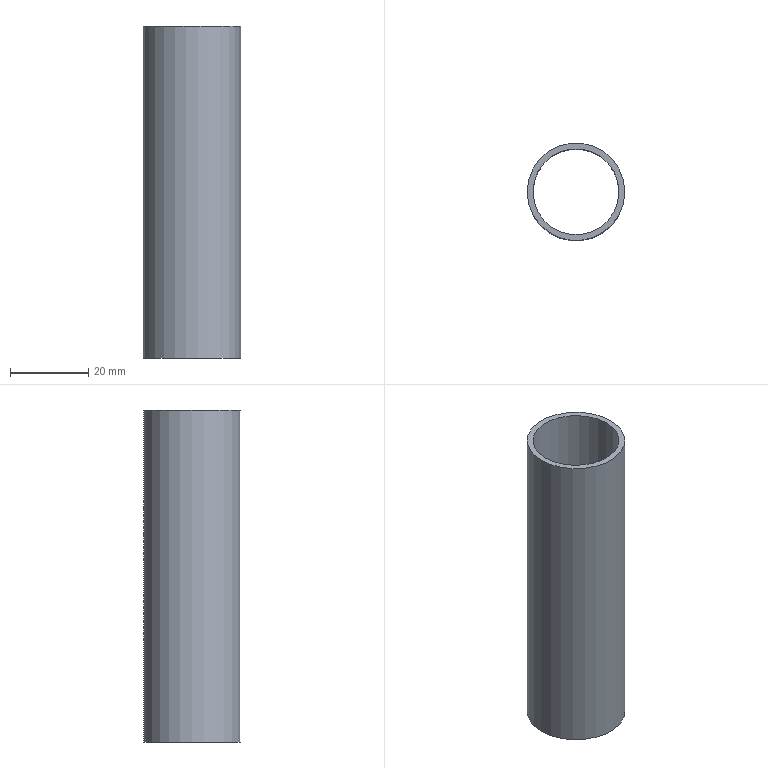Part | STEP file | CMT7E v7 | 1 solid | 4 faces | box 25 x 25 x 85 mm | volume 9413 mm3 | plane 2 | cylinder 2 | commonest cylinder face diameters 22 x1 25 x1
STEP:
#1=CARTESIAN_POINT('',(0.,0.,0.));
#2=DIRECTION('',(0.,0.,1.));
#3=DIRECTION('',(1.,0.,0.));
#4=AXIS2_PLACEMENT_3D('',#1,#2,#3);
#5=CARTESIAN_POINT('',(-80.537,25.309,26.));
#6=VERTEX_POINT('',#5);
#7=CARTESIAN_POINT('',(-69.537,25.309,26.));
#8=DIRECTION('',(0.,0.,-1.));
#9=DIRECTION('',(-1.,0.,0.));
#10=AXIS2_PLACEMENT_3D('',#7,#8,#9);
#11=CIRCLE('',#10,11.);
#12=CARTESIAN_POINT('',(-69.537,25.309,26.));
#13=DIRECTION('',(0.,0.,1.));
#14=DIRECTION('',(-1.,0.,0.));
#15=AXIS2_PLACEMENT_3D('',#12,#13,#14);
#16=PLANE('',#15);
#17=CARTESIAN_POINT('',(11.,0.));
#18=CARTESIAN_POINT('',(11.,-19.053));
#19=CARTESIAN_POINT('',(-5.5,-9.526));
#20=CARTESIAN_POINT('',(-22.,0.));
#21=CARTESIAN_POINT('',(-5.5,9.526));
#22=CARTESIAN_POINT('',(11.,19.053));
#23=CARTESIAN_POINT('',(11.,0.));
#24=(BOUNDED_CURVE()B_SPLINE_CURVE(2,(#17,#18,#19,#20,#21,#22,#23),.UNSPECIFIED.,.T.,.F.)B_SPLINE_CURVE_WITH_KNOTS((1,2,2,2,2,1),(-2.094,0.,2.094,4.189,6.283,8.378),.UNSPECIFIED.)CURVE()GEOMETRIC_REPRESENTATION_ITEM()RATIONAL_B_SPLINE_CURVE((1.,0.5,1.,0.5,1.,0.5,1.))REPRESENTATION_ITEM(''));
#25=(GEOMETRIC_REPRESENTATION_CONTEXT(2)PARAMETRIC_REPRESENTATION_CONTEXT()REPRESENTATION_CONTEXT('',''));
#26=DEFINITIONAL_REPRESENTATION('',(#24),#25);
#27=PCURVE('',#16,#26);
#28=CARTESIAN_POINT('',(-69.537,25.309,26.));
#29=DIRECTION('',(0.,0.,1.));
#30=DIRECTION('',(-1.,0.,0.));
#31=AXIS2_PLACEMENT_3D('',#28,#29,#30);
#32=CYLINDRICAL_SURFACE('',#31,11.);
#33=CARTESIAN_POINT('',(6.283,0.));
#34=DIRECTION('',(-1.,0.));
#35=VECTOR('',#34,1.);
#36=LINE('',#33,#35);
#37=(GEOMETRIC_REPRESENTATION_CONTEXT(2)PARAMETRIC_REPRESENTATION_CONTEXT()REPRESENTATION_CONTEXT('',''));
#38=DEFINITIONAL_REPRESENTATION('',(#36),#37);
#39=PCURVE('',#32,#38);
#40=SURFACE_CURVE('',#11,(#27,#39),.PCURVE_S1.);
#41=EDGE_CURVE('',#6,#6,#40,.T.);
#42=ORIENTED_EDGE('',*,*,#41,.F.);
#43=EDGE_LOOP('',(#42));
#44=FACE_BOUND('',#43,.T.);
#45=CARTESIAN_POINT('',(-82.037,25.309,26.));
#46=VERTEX_POINT('',#45);
#47=CARTESIAN_POINT('',(-69.537,25.309,26.));
#48=DIRECTION('',(0.,0.,1.));
#49=DIRECTION('',(-1.,0.,0.));
#50=AXIS2_PLACEMENT_3D('',#47,#48,#49);
#51=CIRCLE('',#50,12.5);
#52=CARTESIAN_POINT('',(0.,0.));
#53=DIRECTION('',(1.,0.));
#54=AXIS2_PLACEMENT_2D('',#52,#53);
#55=CIRCLE('',#54,12.5);
#56=(GEOMETRIC_REPRESENTATION_CONTEXT(2)PARAMETRIC_REPRESENTATION_CONTEXT()REPRESENTATION_CONTEXT('',''));
#57=DEFINITIONAL_REPRESENTATION('',(#55),#56);
#58=PCURVE('',#16,#57);
#59=CARTESIAN_POINT('',(-69.537,25.309,26.));
#60=DIRECTION('',(0.,0.,1.));
#61=DIRECTION('',(-1.,0.,0.));
#62=AXIS2_PLACEMENT_3D('',#59,#60,#61);
#63=CYLINDRICAL_SURFACE('',#62,12.5);
#64=CARTESIAN_POINT('',(0.,0.));
#65=DIRECTION('',(1.,0.));
#66=VECTOR('',#65,1.);
#67=LINE('',#64,#66);
#68=(GEOMETRIC_REPRESENTATION_CONTEXT(2)PARAMETRIC_REPRESENTATION_CONTEXT()REPRESENTATION_CONTEXT('',''));
#69=DEFINITIONAL_REPRESENTATION('',(#67),#68);
#70=PCURVE('',#63,#69);
#71=SURFACE_CURVE('',#51,(#58,#70),.PCURVE_S1.);
#72=EDGE_CURVE('',#46,#46,#71,.T.);
#73=ORIENTED_EDGE('',*,*,#72,.F.);
#74=EDGE_LOOP('',(#73));
#75=FACE_BOUND('',#74,.T.);
#76=ADVANCED_FACE('',(#44,#75),#16,.F.);
#77=CARTESIAN_POINT('',(-80.537,25.309,111.));
#78=VERTEX_POINT('',#77);
#79=CARTESIAN_POINT('',(-69.537,25.309,111.));
#80=DIRECTION('',(0.,0.,-1.));
#81=DIRECTION('',(-1.,0.,0.));
#82=AXIS2_PLACEMENT_3D('',#79,#80,#81);
#83=CIRCLE('',#82,11.);
#84=CARTESIAN_POINT('',(-69.537,25.309,111.));
#85=DIRECTION('',(0.,0.,1.));
#86=DIRECTION('',(-1.,0.,0.));
#87=AXIS2_PLACEMENT_3D('',#84,#85,#86);
#88=PLANE('',#87);
#89=CARTESIAN_POINT('',(11.,0.));
#90=CARTESIAN_POINT('',(11.,-19.053));
#91=CARTESIAN_POINT('',(-5.5,-9.526));
#92=CARTESIAN_POINT('',(-22.,0.));
#93=CARTESIAN_POINT('',(-5.5,9.526));
#94=CARTESIAN_POINT('',(11.,19.053));
#95=CARTESIAN_POINT('',(11.,0.));
#96=(BOUNDED_CURVE()B_SPLINE_CURVE(2,(#89,#90,#91,#92,#93,#94,#95),.UNSPECIFIED.,.T.,.F.)B_SPLINE_CURVE_WITH_KNOTS((1,2,2,2,2,1),(-2.094,0.,2.094,4.189,6.283,8.378),.UNSPECIFIED.)CURVE()GEOMETRIC_REPRESENTATION_ITEM()RATIONAL_B_SPLINE_CURVE((1.,0.5,1.,0.5,1.,0.5,1.))REPRESENTATION_ITEM(''));
#97=(GEOMETRIC_REPRESENTATION_CONTEXT(2)PARAMETRIC_REPRESENTATION_CONTEXT()REPRESENTATION_CONTEXT('',''));
#98=DEFINITIONAL_REPRESENTATION('',(#96),#97);
#99=PCURVE('',#88,#98);
#100=CARTESIAN_POINT('',(6.283,85.));
#101=DIRECTION('',(-1.,0.));
#102=VECTOR('',#101,1.);
#103=LINE('',#100,#102);
#104=(GEOMETRIC_REPRESENTATION_CONTEXT(2)PARAMETRIC_REPRESENTATION_CONTEXT()REPRESENTATION_CONTEXT('',''));
#105=DEFINITIONAL_REPRESENTATION('',(#103),#104);
#106=PCURVE('',#32,#105);
#107=SURFACE_CURVE('',#83,(#99,#106),.PCURVE_S1.);
#108=EDGE_CURVE('',#78,#78,#107,.T.);
#109=ORIENTED_EDGE('',*,*,#108,.T.);
#110=EDGE_LOOP('',(#109));
#111=FACE_BOUND('',#110,.T.);
#112=CARTESIAN_POINT('',(-82.037,25.309,111.));
#113=VERTEX_POINT('',#112);
#114=CARTESIAN_POINT('',(-69.537,25.309,111.));
#115=DIRECTION('',(0.,0.,1.));
#116=DIRECTION('',(-1.,0.,0.));
#117=AXIS2_PLACEMENT_3D('',#114,#115,#116);
#118=CIRCLE('',#117,12.5);
#119=CARTESIAN_POINT('',(0.,0.));
#120=DIRECTION('',(1.,0.));
#121=AXIS2_PLACEMENT_2D('',#119,#120);
#122=CIRCLE('',#121,12.5);
#123=(GEOMETRIC_REPRESENTATION_CONTEXT(2)PARAMETRIC_REPRESENTATION_CONTEXT()REPRESENTATION_CONTEXT('',''));
#124=DEFINITIONAL_REPRESENTATION('',(#122),#123);
#125=PCURVE('',#88,#124);
#126=CARTESIAN_POINT('',(0.,85.));
#127=DIRECTION('',(1.,0.));
#128=VECTOR('',#127,1.);
#129=LINE('',#126,#128);
#130=(GEOMETRIC_REPRESENTATION_CONTEXT(2)PARAMETRIC_REPRESENTATION_CONTEXT()REPRESENTATION_CONTEXT('',''));
#131=DEFINITIONAL_REPRESENTATION('',(#129),#130);
#132=PCURVE('',#63,#131);
#133=SURFACE_CURVE('',#118,(#125,#132),.PCURVE_S1.);
#134=EDGE_CURVE('',#113,#113,#133,.T.);
#135=ORIENTED_EDGE('',*,*,#134,.T.);
#136=EDGE_LOOP('',(#135));
#137=FACE_BOUND('',#136,.T.);
#138=ADVANCED_FACE('',(#111,#137),#88,.T.);
#139=ORIENTED_EDGE('',*,*,#72,.T.);
#140=CARTESIAN_POINT('',(-82.037,25.309,26.));
#141=CARTESIAN_POINT('',(-82.037,25.309,111.));
#142=B_SPLINE_CURVE_WITH_KNOTS('',1,(#140,#141),.UNSPECIFIED.,.F.,.F.,(2,2),(0.,85.),.PIECEWISE_BEZIER_KNOTS.);
#143=CARTESIAN_POINT('',(6.283,0.));
#144=DIRECTION('',(0.,1.));
#145=VECTOR('',#144,1.);
#146=LINE('',#143,#145);
#147=(GEOMETRIC_REPRESENTATION_CONTEXT(2)PARAMETRIC_REPRESENTATION_CONTEXT()REPRESENTATION_CONTEXT('',''));
#148=DEFINITIONAL_REPRESENTATION('',(#146),#147);
#149=PCURVE('',#63,#148);
#150=CARTESIAN_POINT('',(0.,0.));
#151=DIRECTION('',(0.,1.));
#152=VECTOR('',#151,1.);
#153=LINE('',#150,#152);
#154=(GEOMETRIC_REPRESENTATION_CONTEXT(2)PARAMETRIC_REPRESENTATION_CONTEXT()REPRESENTATION_CONTEXT('',''));
#155=DEFINITIONAL_REPRESENTATION('',(#153),#154);
#156=PCURVE('',#63,#155);
#157=SEAM_CURVE('',#142,(#149,#156),.PCURVE_S1.);
#158=EDGE_CURVE('',#46,#113,#157,.T.);
#159=ORIENTED_EDGE('',*,*,#158,.T.);
#160=ORIENTED_EDGE('',*,*,#134,.F.);
#161=ORIENTED_EDGE('',*,*,#158,.F.);
#162=EDGE_LOOP('',(#139,#159,#160,#161));
#163=FACE_BOUND('',#162,.T.);
#164=ADVANCED_FACE('',(#163),#63,.T.);
#165=ORIENTED_EDGE('',*,*,#41,.F.);
#166=CARTESIAN_POINT('',(-80.537,25.309,26.));
#167=CARTESIAN_POINT('',(-80.537,25.309,111.));
#168=B_SPLINE_CURVE_WITH_KNOTS('',1,(#166,#167),.UNSPECIFIED.,.F.,.F.,(2,2),(0.,85.),.PIECEWISE_BEZIER_KNOTS.);
#169=CARTESIAN_POINT('',(6.283,0.));
#170=DIRECTION('',(0.,1.));
#171=VECTOR('',#170,1.);
#172=LINE('',#169,#171);
#173=(GEOMETRIC_REPRESENTATION_CONTEXT(2)PARAMETRIC_REPRESENTATION_CONTEXT()REPRESENTATION_CONTEXT('',''));
#174=DEFINITIONAL_REPRESENTATION('',(#172),#173);
#175=PCURVE('',#32,#174);
#176=CARTESIAN_POINT('',(0.,0.));
#177=DIRECTION('',(0.,1.));
#178=VECTOR('',#177,1.);
#179=LINE('',#176,#178);
#180=(GEOMETRIC_REPRESENTATION_CONTEXT(2)PARAMETRIC_REPRESENTATION_CONTEXT()REPRESENTATION_CONTEXT('',''));
#181=DEFINITIONAL_REPRESENTATION('',(#179),#180);
#182=PCURVE('',#32,#181);
#183=SEAM_CURVE('',#168,(#175,#182),.PCURVE_S1.);
#184=EDGE_CURVE('',#6,#78,#183,.T.);
#185=ORIENTED_EDGE('',*,*,#184,.T.);
#186=ORIENTED_EDGE('',*,*,#108,.T.);
#187=ORIENTED_EDGE('',*,*,#184,.F.);
#188=EDGE_LOOP('',(#165,#185,#186,#187));
#189=FACE_BOUND('',#188,.F.);
#190=ADVANCED_FACE('',(#189),#32,.F.);
#191=CLOSED_SHELL('',(#76,#138,#164,#190));
#192=MANIFOLD_SOLID_BREP('',#191);
#193=(LENGTH_UNIT()NAMED_UNIT(*)SI_UNIT(.MILLI.,.METRE.));
#194=UNCERTAINTY_MEASURE_WITH_UNIT(LENGTH_MEASURE(0.0000001),#193,'','');
#195=(NAMED_UNIT(*)PLANE_ANGLE_UNIT()SI_UNIT($,.RADIAN.));
#196=(NAMED_UNIT(*)SI_UNIT($,.STERADIAN.)SOLID_ANGLE_UNIT());
#197=(GEOMETRIC_REPRESENTATION_CONTEXT(3)GLOBAL_UNCERTAINTY_ASSIGNED_CONTEXT((#194))GLOBAL_UNIT_ASSIGNED_CONTEXT((#193,#195,#196))REPRESENTATION_CONTEXT('',''));
#198=ADVANCED_BREP_SHAPE_REPRESENTATION('',(#4,#192),#197);